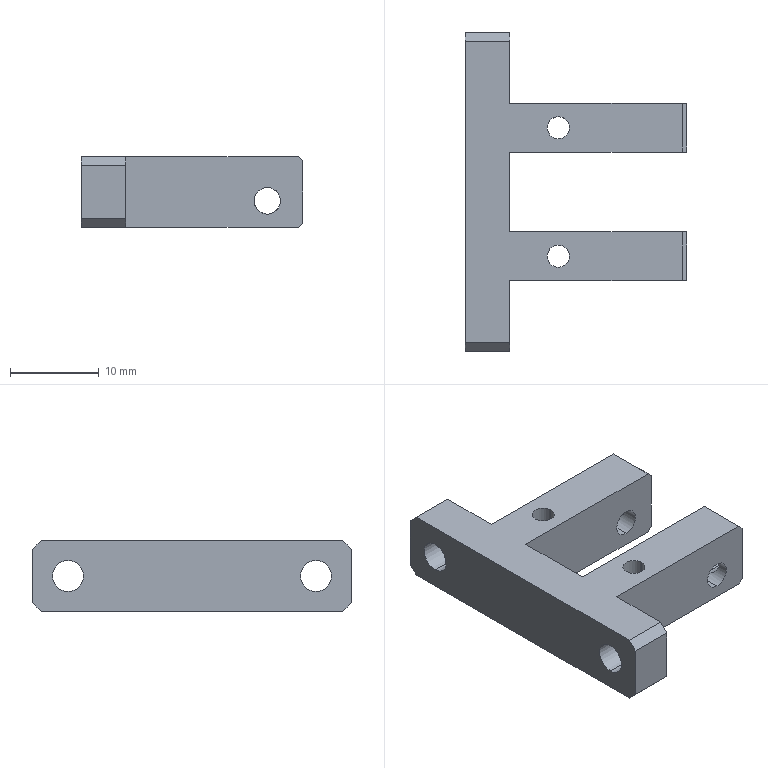Part | NX | features BREP 1 | 1 solid | 48 faces | box 25 x 36 x 8 mm | volume 2909 mm3 | cylinder 22 | plane 22 | cone 4 | commonest cylinder face diameters 2.5 x14 3 x4 3.5 x4